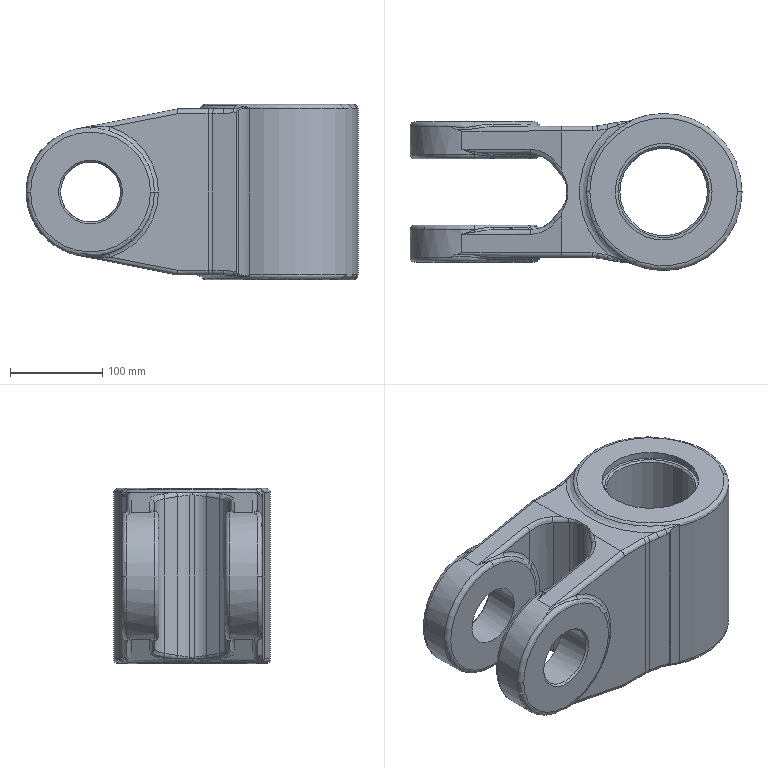Part | SolidWorks | features Fillet 14, ICE 11, Chamfer 4, MirrorPattern 2, Extrusion 1 | 1 solid | 147 faces | box 360 x 170 x 190 mm | volume 5382355 mm3 | spline 42 | cylinder 42 | torus 28 | plane 27 | cone 8 | commonest cylinder face diameters 10 x20 60 x6 65 x4 105 x4 40 x2 95 x2